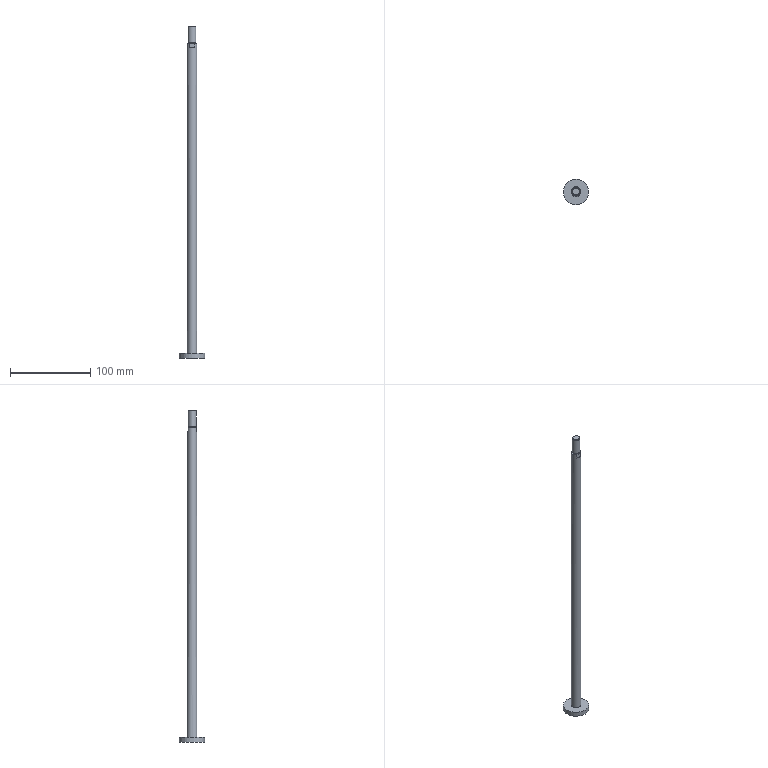Part | STEP file | 163314 DNC-32-320-PPV-A---(FESTO)_HASTE | 1 solid | 13 faces | box 32 x 32 x 415 mm | volume 50245 mm3 | plane 8 | cylinder 3 | cone 2 | commonest cylinder face diameters 10 x1 12 x1 32 x1
STEP:
#1=CARTESIAN_POINT('',(0.,0.,0.));
#2=DIRECTION('',(0.,0.,1.));
#3=DIRECTION('',(1.,0.,0.));
#4=AXIS2_PLACEMENT_3D('',#1,#2,#3);
#5=CARTESIAN_POINT('',(0.,-16.,-361.));
#6=VERTEX_POINT('',#5);
#7=CARTESIAN_POINT('',(0.,0.,-361.));
#8=DIRECTION('',(0.,0.,-1.));
#9=DIRECTION('',(1.,0.,0.));
#10=AXIS2_PLACEMENT_3D('',#7,#8,#9);
#11=CIRCLE('',#10,16.);
#12=CARTESIAN_POINT('',(0.,0.,-364.));
#13=DIRECTION('',(0.,0.,-1.));
#14=DIRECTION('',(0.,-1.,0.));
#15=AXIS2_PLACEMENT_3D('',#12,#13,#14);
#16=CYLINDRICAL_SURFACE('',#15,16.);
#17=CARTESIAN_POINT('',(-1.571,-3.));
#18=DIRECTION('',(1.,0.));
#19=VECTOR('',#18,1.);
#20=LINE('',#17,#19);
#21=(GEOMETRIC_REPRESENTATION_CONTEXT(2)PARAMETRIC_REPRESENTATION_CONTEXT()REPRESENTATION_CONTEXT('',''));
#22=DEFINITIONAL_REPRESENTATION('',(#20),#21);
#23=PCURVE('',#16,#22);
#24=CARTESIAN_POINT('',(0.,9.5,-361.));
#25=DIRECTION('',(0.,0.,1.));
#26=DIRECTION('',(1.,0.,0.));
#27=AXIS2_PLACEMENT_3D('',#24,#25,#26);
#28=PLANE('',#27);
#29=CARTESIAN_POINT('',(16.,-9.5));
#30=CARTESIAN_POINT('',(16.,-37.213));
#31=CARTESIAN_POINT('',(-8.,-23.356));
#32=CARTESIAN_POINT('',(-32.,-9.5));
#33=CARTESIAN_POINT('',(-8.,4.356));
#34=CARTESIAN_POINT('',(16.,18.213));
#35=CARTESIAN_POINT('',(16.,-9.5));
#36=(BOUNDED_CURVE()B_SPLINE_CURVE(2,(#29,#30,#31,#32,#33,#34,#35),.UNSPECIFIED.,.T.,.F.)B_SPLINE_CURVE_WITH_KNOTS((1,2,2,2,2,1),(-2.094,0.,2.094,4.189,6.283,8.378),.UNSPECIFIED.)CURVE()GEOMETRIC_REPRESENTATION_ITEM()RATIONAL_B_SPLINE_CURVE((1.,0.5,1.,0.5,1.,0.5,1.))REPRESENTATION_ITEM(''));
#37=(GEOMETRIC_REPRESENTATION_CONTEXT(2)PARAMETRIC_REPRESENTATION_CONTEXT()REPRESENTATION_CONTEXT('',''));
#38=DEFINITIONAL_REPRESENTATION('',(#36),#37);
#39=PCURVE('',#28,#38);
#40=SURFACE_CURVE('',#11,(#23,#39),.PCURVE_S1.);
#41=EDGE_CURVE('',#6,#6,#40,.T.);
#42=ORIENTED_EDGE('',*,*,#41,.T.);
#43=CARTESIAN_POINT('',(0.,-16.,-367.));
#44=VERTEX_POINT('',#43);
#45=CARTESIAN_POINT('',(0.,-16.,-361.));
#46=CARTESIAN_POINT('',(0.,-16.,-367.));
#47=B_SPLINE_CURVE_WITH_KNOTS('',1,(#45,#46),.UNSPECIFIED.,.F.,.F.,(2,2),(-3.,3.),.PIECEWISE_BEZIER_KNOTS.);
#48=CARTESIAN_POINT('',(6.283,0.));
#49=DIRECTION('',(0.,1.));
#50=VECTOR('',#49,1.);
#51=LINE('',#48,#50);
#52=(GEOMETRIC_REPRESENTATION_CONTEXT(2)PARAMETRIC_REPRESENTATION_CONTEXT()REPRESENTATION_CONTEXT('',''));
#53=DEFINITIONAL_REPRESENTATION('',(#51),#52);
#54=PCURVE('',#16,#53);
#55=CARTESIAN_POINT('',(0.,0.));
#56=DIRECTION('',(0.,1.));
#57=VECTOR('',#56,1.);
#58=LINE('',#55,#57);
#59=(GEOMETRIC_REPRESENTATION_CONTEXT(2)PARAMETRIC_REPRESENTATION_CONTEXT()REPRESENTATION_CONTEXT('',''));
#60=DEFINITIONAL_REPRESENTATION('',(#58),#59);
#61=PCURVE('',#16,#60);
#62=SEAM_CURVE('',#47,(#54,#61),.PCURVE_S1.);
#63=EDGE_CURVE('',#6,#44,#62,.T.);
#64=ORIENTED_EDGE('',*,*,#63,.T.);
#65=CARTESIAN_POINT('',(0.,0.,-367.));
#66=DIRECTION('',(0.,0.,-1.));
#67=DIRECTION('',(1.,0.,0.));
#68=AXIS2_PLACEMENT_3D('',#65,#66,#67);
#69=CIRCLE('',#68,16.);
#70=CARTESIAN_POINT('',(-1.571,3.));
#71=DIRECTION('',(1.,0.));
#72=VECTOR('',#71,1.);
#73=LINE('',#70,#72);
#74=(GEOMETRIC_REPRESENTATION_CONTEXT(2)PARAMETRIC_REPRESENTATION_CONTEXT()REPRESENTATION_CONTEXT('',''));
#75=DEFINITIONAL_REPRESENTATION('',(#73),#74);
#76=PCURVE('',#16,#75);
#77=CARTESIAN_POINT('',(0.,8.,-367.));
#78=DIRECTION('',(0.,0.,-1.));
#79=DIRECTION('',(-1.,0.,0.));
#80=AXIS2_PLACEMENT_3D('',#77,#78,#79);
#81=PLANE('',#80);
#82=CARTESIAN_POINT('',(0.,-8.));
#83=DIRECTION('',(-1.,0.));
#84=AXIS2_PLACEMENT_2D('',#82,#83);
#85=CIRCLE('',#84,16.);
#86=(GEOMETRIC_REPRESENTATION_CONTEXT(2)PARAMETRIC_REPRESENTATION_CONTEXT()REPRESENTATION_CONTEXT('',''));
#87=DEFINITIONAL_REPRESENTATION('',(#85),#86);
#88=PCURVE('',#81,#87);
#89=SURFACE_CURVE('',#69,(#76,#88),.PCURVE_S1.);
#90=EDGE_CURVE('',#44,#44,#89,.T.);
#91=ORIENTED_EDGE('',*,*,#90,.F.);
#92=ORIENTED_EDGE('',*,*,#63,.F.);
#93=EDGE_LOOP('',(#42,#64,#91,#92));
#94=FACE_BOUND('',#93,.T.);
#95=ADVANCED_FACE('',(#94),#16,.T.);
#96=ORIENTED_EDGE('',*,*,#90,.T.);
#97=EDGE_LOOP('',(#96));
#98=FACE_BOUND('',#97,.T.);
#99=ADVANCED_FACE('',(#98),#81,.T.);
#100=ORIENTED_EDGE('',*,*,#41,.F.);
#101=EDGE_LOOP('',(#100));
#102=FACE_BOUND('',#101,.T.);
#103=CARTESIAN_POINT('',(0.,-6.,-361.));
#104=VERTEX_POINT('',#103);
#105=CARTESIAN_POINT('',(0.,0.,-361.));
#106=DIRECTION('',(0.,0.,-1.));
#107=DIRECTION('',(0.,1.,0.));
#108=AXIS2_PLACEMENT_3D('',#105,#106,#107);
#109=CIRCLE('',#108,6.);
#110=CARTESIAN_POINT('',(0.,-3.5));
#111=CARTESIAN_POINT('',(10.392,-3.5));
#112=CARTESIAN_POINT('',(5.196,-12.5));
#113=CARTESIAN_POINT('',(0.,-21.5));
#114=CARTESIAN_POINT('',(-5.196,-12.5));
#115=CARTESIAN_POINT('',(-10.392,-3.5));
#116=CARTESIAN_POINT('',(0.,-3.5));
#117=(BOUNDED_CURVE()B_SPLINE_CURVE(2,(#110,#111,#112,#113,#114,#115,#116),.UNSPECIFIED.,.T.,.F.)B_SPLINE_CURVE_WITH_KNOTS((1,2,2,2,2,1),(-2.094,0.,2.094,4.189,6.283,8.378),.UNSPECIFIED.)CURVE()GEOMETRIC_REPRESENTATION_ITEM()RATIONAL_B_SPLINE_CURVE((1.,0.5,1.,0.5,1.,0.5,1.))REPRESENTATION_ITEM(''));
#118=(GEOMETRIC_REPRESENTATION_CONTEXT(2)PARAMETRIC_REPRESENTATION_CONTEXT()REPRESENTATION_CONTEXT('',''));
#119=DEFINITIONAL_REPRESENTATION('',(#117),#118);
#120=PCURVE('',#28,#119);
#121=CARTESIAN_POINT('',(0.,0.,-170.45));
#122=DIRECTION('',(0.,0.,-1.));
#123=DIRECTION('',(0.,-1.,0.));
#124=AXIS2_PLACEMENT_3D('',#121,#122,#123);
#125=CYLINDRICAL_SURFACE('',#124,6.);
#126=CARTESIAN_POINT('',(-3.142,190.55));
#127=DIRECTION('',(1.,0.));
#128=VECTOR('',#127,1.);
#129=LINE('',#126,#128);
#130=(GEOMETRIC_REPRESENTATION_CONTEXT(2)PARAMETRIC_REPRESENTATION_CONTEXT()REPRESENTATION_CONTEXT('',''));
#131=DEFINITIONAL_REPRESENTATION('',(#129),#130);
#132=PCURVE('',#125,#131);
#133=SURFACE_CURVE('',#109,(#120,#132),.PCURVE_S1.);
#134=EDGE_CURVE('',#104,#104,#133,.T.);
#135=ORIENTED_EDGE('',*,*,#134,.T.);
#136=EDGE_LOOP('',(#135));
#137=FACE_BOUND('',#136,.T.);
#138=ADVANCED_FACE('',(#102,#137),#28,.T.);
#139=CARTESIAN_POINT('',(3.317,-5.,21.));
#140=VERTEX_POINT('',#139);
#141=CARTESIAN_POINT('',(0.,-6.,21.));
#142=VERTEX_POINT('',#141);
#143=CARTESIAN_POINT('',(0.,0.,21.));
#144=DIRECTION('',(0.,0.,-1.));
#145=DIRECTION('',(-0.5528,-0.8333,0.));
#146=AXIS2_PLACEMENT_3D('',#143,#144,#145);
#147=CIRCLE('',#146,6.);
#148=CARTESIAN_POINT('',(0.5857,-191.45));
#149=DIRECTION('',(1.,0.000000001));
#150=VECTOR('',#149,1.);
#151=LINE('',#148,#150);
#152=(GEOMETRIC_REPRESENTATION_CONTEXT(2)PARAMETRIC_REPRESENTATION_CONTEXT()REPRESENTATION_CONTEXT('',''));
#153=DEFINITIONAL_REPRESENTATION('',(#151),#152);
#154=PCURVE('',#125,#153);
#155=CARTESIAN_POINT('',(0.,0.,21.));
#156=DIRECTION('',(0.,0.,1.));
#157=DIRECTION('',(1.,0.,0.));
#158=AXIS2_PLACEMENT_3D('',#155,#156,#157);
#159=PLANE('',#158);
#160=CARTESIAN_POINT('',(-3.317,-5.));
#161=CARTESIAN_POINT('',(-11.977,0.7446));
#162=CARTESIAN_POINT('',(-2.672,5.372));
#163=CARTESIAN_POINT('',(6.633,10.));
#164=CARTESIAN_POINT('',(5.988,-0.3723));
#165=CARTESIAN_POINT('',(5.344,-10.745));
#166=CARTESIAN_POINT('',(-3.317,-5.));
#167=(BOUNDED_CURVE()B_SPLINE_CURVE(2,(#160,#161,#162,#163,#164,#165,#166),.UNSPECIFIED.,.T.,.F.)B_SPLINE_CURVE_WITH_KNOTS((1,2,2,2,2,1),(-2.094,0.,2.094,4.189,6.283,8.378),.UNSPECIFIED.)CURVE()GEOMETRIC_REPRESENTATION_ITEM()RATIONAL_B_SPLINE_CURVE((1.,0.5,1.,0.5,1.,0.5,1.))REPRESENTATION_ITEM(''));
#168=(GEOMETRIC_REPRESENTATION_CONTEXT(2)PARAMETRIC_REPRESENTATION_CONTEXT()REPRESENTATION_CONTEXT('',''));
#169=DEFINITIONAL_REPRESENTATION('',(#167),#168);
#170=PCURVE('',#159,#169);
#171=SURFACE_CURVE('',#147,(#154,#170),.PCURVE_S1.);
#172=EDGE_CURVE('',#140,#142,#171,.T.);
#173=ORIENTED_EDGE('',*,*,#172,.T.);
#174=CARTESIAN_POINT('',(0.,-6.,21.));
#175=CARTESIAN_POINT('',(0.,-6.,-361.));
#176=B_SPLINE_CURVE_WITH_KNOTS('',1,(#174,#175),.UNSPECIFIED.,.F.,.F.,(2,2),(-191.45,190.55),.PIECEWISE_BEZIER_KNOTS.);
#177=CARTESIAN_POINT('',(6.283,0.));
#178=DIRECTION('',(0.,1.));
#179=VECTOR('',#178,1.);
#180=LINE('',#177,#179);
#181=(GEOMETRIC_REPRESENTATION_CONTEXT(2)PARAMETRIC_REPRESENTATION_CONTEXT()REPRESENTATION_CONTEXT('',''));
#182=DEFINITIONAL_REPRESENTATION('',(#180),#181);
#183=PCURVE('',#125,#182);
#184=CARTESIAN_POINT('',(0.,0.));
#185=DIRECTION('',(0.,1.));
#186=VECTOR('',#185,1.);
#187=LINE('',#184,#186);
#188=(GEOMETRIC_REPRESENTATION_CONTEXT(2)PARAMETRIC_REPRESENTATION_CONTEXT()REPRESENTATION_CONTEXT('',''));
#189=DEFINITIONAL_REPRESENTATION('',(#187),#188);
#190=PCURVE('',#125,#189);
#191=SEAM_CURVE('',#176,(#183,#190),.PCURVE_S1.);
#192=EDGE_CURVE('',#142,#104,#191,.T.);
#193=ORIENTED_EDGE('',*,*,#192,.T.);
#194=ORIENTED_EDGE('',*,*,#134,.F.);
#195=ORIENTED_EDGE('',*,*,#192,.F.);
#196=CARTESIAN_POINT('',(-3.317,-5.,21.));
#197=VERTEX_POINT('',#196);
#198=CARTESIAN_POINT('',(0.,0.,21.));
#199=DIRECTION('',(0.,0.,-1.));
#200=DIRECTION('',(-0.5528,-0.8333,0.));
#201=AXIS2_PLACEMENT_3D('',#198,#199,#200);
#202=CIRCLE('',#201,6.);
#203=CARTESIAN_POINT('',(-5.697,-191.45));
#204=DIRECTION('',(1.,0.000000001));
#205=VECTOR('',#204,1.);
#206=LINE('',#203,#205);
#207=(GEOMETRIC_REPRESENTATION_CONTEXT(2)PARAMETRIC_REPRESENTATION_CONTEXT()REPRESENTATION_CONTEXT('',''));
#208=DEFINITIONAL_REPRESENTATION('',(#206),#207);
#209=PCURVE('',#125,#208);
#210=CARTESIAN_POINT('',(-3.317,-5.));
#211=CARTESIAN_POINT('',(-11.977,0.7446));
#212=CARTESIAN_POINT('',(-2.672,5.372));
#213=CARTESIAN_POINT('',(6.633,10.));
#214=CARTESIAN_POINT('',(5.988,-0.3723));
#215=CARTESIAN_POINT('',(5.344,-10.745));
#216=CARTESIAN_POINT('',(-3.317,-5.));
#217=(BOUNDED_CURVE()B_SPLINE_CURVE(2,(#210,#211,#212,#213,#214,#215,#216),.UNSPECIFIED.,.T.,.F.)B_SPLINE_CURVE_WITH_KNOTS((1,2,2,2,2,1),(-2.094,0.,2.094,4.189,6.283,8.378),.UNSPECIFIED.)CURVE()GEOMETRIC_REPRESENTATION_ITEM()RATIONAL_B_SPLINE_CURVE((1.,0.5,1.,0.5,1.,0.5,1.))REPRESENTATION_ITEM(''));
#218=(GEOMETRIC_REPRESENTATION_CONTEXT(2)PARAMETRIC_REPRESENTATION_CONTEXT()REPRESENTATION_CONTEXT('',''));
#219=DEFINITIONAL_REPRESENTATION('',(#217),#218);
#220=PCURVE('',#159,#219);
#221=SURFACE_CURVE('',#202,(#209,#220),.PCURVE_S1.);
#222=EDGE_CURVE('',#142,#197,#221,.T.);
#223=ORIENTED_EDGE('',*,*,#222,.T.);
#224=CARTESIAN_POINT('',(-3.317,-5.,26.));
#225=VERTEX_POINT('',#224);
#226=CARTESIAN_POINT('',(-3.317,-5.,26.));
#227=DIRECTION('',(0.,0.,-1.));
#228=VECTOR('',#227,1.);
#229=LINE('',#226,#228);
#230=CARTESIAN_POINT('',(0.5857,-196.45));
#231=DIRECTION('',(0.,1.));
#232=VECTOR('',#231,1.);
#233=LINE('',#230,#232);
#234=(GEOMETRIC_REPRESENTATION_CONTEXT(2)PARAMETRIC_REPRESENTATION_CONTEXT()REPRESENTATION_CONTEXT('',''));
#235=DEFINITIONAL_REPRESENTATION('',(#233),#234);
#236=PCURVE('',#125,#235);
#237=CARTESIAN_POINT('',(12.,-5.,31.));
#238=DIRECTION('',(0.,1.,0.));
#239=DIRECTION('',(0.,0.,1.));
#240=AXIS2_PLACEMENT_3D('',#237,#238,#239);
#241=PLANE('',#240);
#242=CARTESIAN_POINT('',(-5.,-15.317));
#243=DIRECTION('',(-1.,0.));
#244=VECTOR('',#243,1.);
#245=LINE('',#242,#244);
#246=(GEOMETRIC_REPRESENTATION_CONTEXT(2)PARAMETRIC_REPRESENTATION_CONTEXT()REPRESENTATION_CONTEXT('',''));
#247=DEFINITIONAL_REPRESENTATION('',(#245),#246);
#248=PCURVE('',#241,#247);
#249=SURFACE_CURVE('',#229,(#236,#248),.PCURVE_S1.);
#250=EDGE_CURVE('',#225,#197,#249,.T.);
#251=ORIENTED_EDGE('',*,*,#250,.F.);
#252=CARTESIAN_POINT('',(-3.317,5.,26.));
#253=VERTEX_POINT('',#252);
#254=CARTESIAN_POINT('',(0.,0.,26.));
#255=DIRECTION('',(0.,0.,-1.));
#256=DIRECTION('',(1.,0.,0.));
#257=AXIS2_PLACEMENT_3D('',#254,#255,#256);
#258=CIRCLE('',#257,6.);
#259=CARTESIAN_POINT('',(-1.571,-196.45));
#260=DIRECTION('',(1.,0.));
#261=VECTOR('',#260,1.);
#262=LINE('',#259,#261);
#263=(GEOMETRIC_REPRESENTATION_CONTEXT(2)PARAMETRIC_REPRESENTATION_CONTEXT()REPRESENTATION_CONTEXT('',''));
#264=DEFINITIONAL_REPRESENTATION('',(#262),#263);
#265=PCURVE('',#125,#264);
#266=CARTESIAN_POINT('',(0.,3.,26.));
#267=DIRECTION('',(0.,0.,1.));
#268=DIRECTION('',(1.,0.,0.));
#269=AXIS2_PLACEMENT_3D('',#266,#267,#268);
#270=PLANE('',#269);
#271=CARTESIAN_POINT('',(6.,-3.));
#272=CARTESIAN_POINT('',(6.,-13.392));
#273=CARTESIAN_POINT('',(-3.,-8.196));
#274=CARTESIAN_POINT('',(-12.,-3.));
#275=CARTESIAN_POINT('',(-3.,2.196));
#276=CARTESIAN_POINT('',(6.,7.392));
#277=CARTESIAN_POINT('',(6.,-3.));
#278=(BOUNDED_CURVE()B_SPLINE_CURVE(2,(#271,#272,#273,#274,#275,#276,#277),.UNSPECIFIED.,.T.,.F.)B_SPLINE_CURVE_WITH_KNOTS((1,2,2,2,2,1),(-2.094,0.,2.094,4.189,6.283,8.378),.UNSPECIFIED.)CURVE()GEOMETRIC_REPRESENTATION_ITEM()RATIONAL_B_SPLINE_CURVE((1.,0.5,1.,0.5,1.,0.5,1.))REPRESENTATION_ITEM(''));
#279=(GEOMETRIC_REPRESENTATION_CONTEXT(2)PARAMETRIC_REPRESENTATION_CONTEXT()REPRESENTATION_CONTEXT('',''));
#280=DEFINITIONAL_REPRESENTATION('',(#278),#279);
#281=PCURVE('',#270,#280);
#282=SURFACE_CURVE('',#258,(#265,#281),.PCURVE_S1.);
#283=EDGE_CURVE('',#225,#253,#282,.T.);
#284=ORIENTED_EDGE('',*,*,#283,.T.);
#285=CARTESIAN_POINT('',(-3.317,5.,21.));
#286=VERTEX_POINT('',#285);
#287=CARTESIAN_POINT('',(-3.317,5.,26.));
#288=DIRECTION('',(0.,0.,-1.));
#289=VECTOR('',#288,1.);
#290=LINE('',#287,#289);
#291=CARTESIAN_POINT('',(2.556,-196.45));
#292=DIRECTION('',(0.,1.));
#293=VECTOR('',#292,1.);
#294=LINE('',#291,#293);
#295=(GEOMETRIC_REPRESENTATION_CONTEXT(2)PARAMETRIC_REPRESENTATION_CONTEXT()REPRESENTATION_CONTEXT('',''));
#296=DEFINITIONAL_REPRESENTATION('',(#294),#295);
#297=PCURVE('',#125,#296);
#298=CARTESIAN_POINT('',(-12.,5.,31.));
#299=DIRECTION('',(0.,-1.,0.));
#300=DIRECTION('',(0.,0.,-1.));
#301=AXIS2_PLACEMENT_3D('',#298,#299,#300);
#302=PLANE('',#301);
#303=CARTESIAN_POINT('',(5.,8.683));
#304=DIRECTION('',(1.,0.));
#305=VECTOR('',#304,1.);
#306=LINE('',#303,#305);
#307=(GEOMETRIC_REPRESENTATION_CONTEXT(2)PARAMETRIC_REPRESENTATION_CONTEXT()REPRESENTATION_CONTEXT('',''));
#308=DEFINITIONAL_REPRESENTATION('',(#306),#307);
#309=PCURVE('',#302,#308);
#310=SURFACE_CURVE('',#290,(#297,#309),.PCURVE_S1.);
#311=EDGE_CURVE('',#253,#286,#310,.T.);
#312=ORIENTED_EDGE('',*,*,#311,.T.);
#313=CARTESIAN_POINT('',(3.317,5.,21.));
#314=VERTEX_POINT('',#313);
#315=CARTESIAN_POINT('',(0.,0.,21.));
#316=DIRECTION('',(0.,0.,-1.));
#317=DIRECTION('',(1.,0.,0.));
#318=AXIS2_PLACEMENT_3D('',#315,#316,#317);
#319=CIRCLE('',#318,6.);
#320=CARTESIAN_POINT('',(-1.571,-191.45));
#321=DIRECTION('',(1.,0.));
#322=VECTOR('',#321,1.);
#323=LINE('',#320,#322);
#324=(GEOMETRIC_REPRESENTATION_CONTEXT(2)PARAMETRIC_REPRESENTATION_CONTEXT()REPRESENTATION_CONTEXT('',''));
#325=DEFINITIONAL_REPRESENTATION('',(#323),#324);
#326=PCURVE('',#125,#325);
#327=CARTESIAN_POINT('',(0.,0.,21.));
#328=DIRECTION('',(0.,0.,1.));
#329=DIRECTION('',(1.,0.,0.));
#330=AXIS2_PLACEMENT_3D('',#327,#328,#329);
#331=PLANE('',#330);
#332=CARTESIAN_POINT('',(6.,0.));
#333=CARTESIAN_POINT('',(6.,-10.392));
#334=CARTESIAN_POINT('',(-3.,-5.196));
#335=CARTESIAN_POINT('',(-12.,0.));
#336=CARTESIAN_POINT('',(-3.,5.196));
#337=CARTESIAN_POINT('',(6.,10.392));
#338=CARTESIAN_POINT('',(6.,0.));
#339=(BOUNDED_CURVE()B_SPLINE_CURVE(2,(#332,#333,#334,#335,#336,#337,#338),.UNSPECIFIED.,.T.,.F.)B_SPLINE_CURVE_WITH_KNOTS((1,2,2,2,2,1),(-2.094,0.,2.094,4.189,6.283,8.378),.UNSPECIFIED.)CURVE()GEOMETRIC_REPRESENTATION_ITEM()RATIONAL_B_SPLINE_CURVE((1.,0.5,1.,0.5,1.,0.5,1.))REPRESENTATION_ITEM(''));
#340=(GEOMETRIC_REPRESENTATION_CONTEXT(2)PARAMETRIC_REPRESENTATION_CONTEXT()REPRESENTATION_CONTEXT('',''));
#341=DEFINITIONAL_REPRESENTATION('',(#339),#340);
#342=PCURVE('',#331,#341);
#343=SURFACE_CURVE('',#319,(#326,#342),.PCURVE_S1.);
#344=EDGE_CURVE('',#286,#314,#343,.T.);
#345=ORIENTED_EDGE('',*,*,#344,.T.);
#346=CARTESIAN_POINT('',(3.317,5.,26.));
#347=VERTEX_POINT('',#346);
#348=CARTESIAN_POINT('',(3.317,5.,26.));
#349=DIRECTION('',(0.,0.,-1.));
#350=VECTOR('',#349,1.);
#351=LINE('',#348,#350);
#352=CARTESIAN_POINT('',(3.727,-196.45));
#353=DIRECTION('',(0.,1.));
#354=VECTOR('',#353,1.);
#355=LINE('',#352,#354);
#356=(GEOMETRIC_REPRESENTATION_CONTEXT(2)PARAMETRIC_REPRESENTATION_CONTEXT()REPRESENTATION_CONTEXT('',''));
#357=DEFINITIONAL_REPRESENTATION('',(#355),#356);
#358=PCURVE('',#125,#357);
#359=CARTESIAN_POINT('',(5.,15.317));
#360=DIRECTION('',(1.,0.));
#361=VECTOR('',#360,1.);
#362=LINE('',#359,#361);
#363=(GEOMETRIC_REPRESENTATION_CONTEXT(2)PARAMETRIC_REPRESENTATION_CONTEXT()REPRESENTATION_CONTEXT('',''));
#364=DEFINITIONAL_REPRESENTATION('',(#362),#363);
#365=PCURVE('',#302,#364);
#366=SURFACE_CURVE('',#351,(#358,#365),.PCURVE_S1.);
#367=EDGE_CURVE('',#347,#314,#366,.T.);
#368=ORIENTED_EDGE('',*,*,#367,.F.);
#369=CARTESIAN_POINT('',(3.317,-5.,26.));
#370=VERTEX_POINT('',#369);
#371=CARTESIAN_POINT('',(0.,0.,26.));
#372=DIRECTION('',(0.,0.,-1.));
#373=DIRECTION('',(1.,0.,0.));
#374=AXIS2_PLACEMENT_3D('',#371,#372,#373);
#375=CIRCLE('',#374,6.);
#376=CARTESIAN_POINT('',(-1.571,-196.45));
#377=DIRECTION('',(1.,0.));
#378=VECTOR('',#377,1.);
#379=LINE('',#376,#378);
#380=(GEOMETRIC_REPRESENTATION_CONTEXT(2)PARAMETRIC_REPRESENTATION_CONTEXT()REPRESENTATION_CONTEXT('',''));
#381=DEFINITIONAL_REPRESENTATION('',(#379),#380);
#382=PCURVE('',#125,#381);
#383=CARTESIAN_POINT('',(6.,-3.));
#384=CARTESIAN_POINT('',(6.,-13.392));
#385=CARTESIAN_POINT('',(-3.,-8.196));
#386=CARTESIAN_POINT('',(-12.,-3.));
#387=CARTESIAN_POINT('',(-3.,2.196));
#388=CARTESIAN_POINT('',(6.,7.392));
#389=CARTESIAN_POINT('',(6.,-3.));
#390=(BOUNDED_CURVE()B_SPLINE_CURVE(2,(#383,#384,#385,#386,#387,#388,#389),.UNSPECIFIED.,.T.,.F.)B_SPLINE_CURVE_WITH_KNOTS((1,2,2,2,2,1),(-2.094,0.,2.094,4.189,6.283,8.378),.UNSPECIFIED.)CURVE()GEOMETRIC_REPRESENTATION_ITEM()RATIONAL_B_SPLINE_CURVE((1.,0.5,1.,0.5,1.,0.5,1.))REPRESENTATION_ITEM(''));
#391=(GEOMETRIC_REPRESENTATION_CONTEXT(2)PARAMETRIC_REPRESENTATION_CONTEXT()REPRESENTATION_CONTEXT('',''));
#392=DEFINITIONAL_REPRESENTATION('',(#390),#391);
#393=PCURVE('',#270,#392);
#394=SURFACE_CURVE('',#375,(#382,#393),.PCURVE_S1.);
#395=EDGE_CURVE('',#347,#370,#394,.T.);
#396=ORIENTED_EDGE('',*,*,#395,.T.);
#397=CARTESIAN_POINT('',(3.317,-5.,26.));
#398=DIRECTION('',(0.,0.,-1.));
#399=VECTOR('',#398,1.);
#400=LINE('',#397,#399);
#401=CARTESIAN_POINT('',(5.697,-196.45));
#402=DIRECTION('',(0.,1.));
#403=VECTOR('',#402,1.);
#404=LINE('',#401,#403);
#405=(GEOMETRIC_REPRESENTATION_CONTEXT(2)PARAMETRIC_REPRESENTATION_CONTEXT()REPRESENTATION_CONTEXT('',''));
#406=DEFINITIONAL_REPRESENTATION('',(#404),#405);
#407=PCURVE('',#125,#406);
#408=CARTESIAN_POINT('',(-5.,-8.683));
#409=DIRECTION('',(-1.,0.));
#410=VECTOR('',#409,1.);
#411=LINE('',#408,#410);
#412=(GEOMETRIC_REPRESENTATION_CONTEXT(2)PARAMETRIC_REPRESENTATION_CONTEXT()REPRESENTATION_CONTEXT('',''));
#413=DEFINITIONAL_REPRESENTATION('',(#411),#412);
#414=PCURVE('',#241,#413);
#415=SURFACE_CURVE('',#400,(#407,#414),.PCURVE_S1.);
#416=EDGE_CURVE('',#370,#140,#415,.T.);
#417=ORIENTED_EDGE('',*,*,#416,.T.);
#418=EDGE_LOOP('',(#173,#193,#194,#195,#223,#251,#284,#312,#345,#368,#396,#417));
#419=FACE_BOUND('',#418,.T.);
#420=ADVANCED_FACE('',(#419),#125,.T.);
#421=ORIENTED_EDGE('',*,*,#172,.F.);
#422=CARTESIAN_POINT('',(3.317,-5.,21.));
#423=DIRECTION('',(-1.,0.,0.));
#424=VECTOR('',#423,1.);
#425=LINE('',#422,#424);
#426=CARTESIAN_POINT('',(3.317,-5.));
#427=DIRECTION('',(-1.,0.));
#428=VECTOR('',#427,1.);
#429=LINE('',#426,#428);
#430=(GEOMETRIC_REPRESENTATION_CONTEXT(2)PARAMETRIC_REPRESENTATION_CONTEXT()REPRESENTATION_CONTEXT('',''));
#431=DEFINITIONAL_REPRESENTATION('',(#429),#430);
#432=PCURVE('',#159,#431);
#433=CARTESIAN_POINT('',(-10.,-8.683));
#434=DIRECTION('',(0.,-1.));
#435=VECTOR('',#434,1.);
#436=LINE('',#433,#435);
#437=(GEOMETRIC_REPRESENTATION_CONTEXT(2)PARAMETRIC_REPRESENTATION_CONTEXT()REPRESENTATION_CONTEXT('',''));
#438=DEFINITIONAL_REPRESENTATION('',(#436),#437);
#439=PCURVE('',#241,#438);
#440=SURFACE_CURVE('',#425,(#432,#439),.PCURVE_S1.);
#441=EDGE_CURVE('',#140,#197,#440,.T.);
#442=ORIENTED_EDGE('',*,*,#441,.T.);
#443=ORIENTED_EDGE('',*,*,#222,.F.);
#444=EDGE_LOOP('',(#421,#442,#443));
#445=FACE_BOUND('',#444,.T.);
#446=ADVANCED_FACE('',(#445),#159,.T.);
#447=ORIENTED_EDGE('',*,*,#250,.T.);
#448=ORIENTED_EDGE('',*,*,#441,.F.);
#449=ORIENTED_EDGE('',*,*,#416,.F.);
#450=CARTESIAN_POINT('',(-3.317,-5.,26.));
#451=DIRECTION('',(1.,0.,0.));
#452=VECTOR('',#451,1.);
#453=LINE('',#450,#452);
#454=CARTESIAN_POINT('',(-5.,-15.317));
#455=DIRECTION('',(0.,1.));
#456=VECTOR('',#455,1.);
#457=LINE('',#454,#456);
#458=(GEOMETRIC_REPRESENTATION_CONTEXT(2)PARAMETRIC_REPRESENTATION_CONTEXT()REPRESENTATION_CONTEXT('',''));
#459=DEFINITIONAL_REPRESENTATION('',(#457),#458);
#460=PCURVE('',#241,#459);
#461=CARTESIAN_POINT('',(-3.317,-8.));
#462=DIRECTION('',(1.,0.));
#463=VECTOR('',#462,1.);
#464=LINE('',#461,#463);
#465=(GEOMETRIC_REPRESENTATION_CONTEXT(2)PARAMETRIC_REPRESENTATION_CONTEXT()REPRESENTATION_CONTEXT('',''));
#466=DEFINITIONAL_REPRESENTATION('',(#464),#465);
#467=PCURVE('',#270,#466);
#468=SURFACE_CURVE('',#453,(#460,#467),.PCURVE_S1.);
#469=EDGE_CURVE('',#225,#370,#468,.T.);
#470=ORIENTED_EDGE('',*,*,#469,.F.);
#471=EDGE_LOOP('',(#447,#448,#449,#470));
#472=FACE_BOUND('',#471,.T.);
#473=ADVANCED_FACE('',(#472),#241,.F.);
#474=ORIENTED_EDGE('',*,*,#469,.T.);
#475=ORIENTED_EDGE('',*,*,#395,.F.);
#476=CARTESIAN_POINT('',(3.317,5.,26.));
#477=DIRECTION('',(-1.,0.,0.));
#478=VECTOR('',#477,1.);
#479=LINE('',#476,#478);
#480=CARTESIAN_POINT('',(3.317,2.));
#481=DIRECTION('',(-1.,0.));
#482=VECTOR('',#481,1.);
#483=LINE('',#480,#482);
#484=(GEOMETRIC_REPRESENTATION_CONTEXT(2)PARAMETRIC_REPRESENTATION_CONTEXT()REPRESENTATION_CONTEXT('',''));
#485=DEFINITIONAL_REPRESENTATION('',(#483),#484);
#486=PCURVE('',#270,#485);
#487=CARTESIAN_POINT('',(5.,15.317));
#488=DIRECTION('',(0.,-1.));
#489=VECTOR('',#488,1.);
#490=LINE('',#487,#489);
#491=(GEOMETRIC_REPRESENTATION_CONTEXT(2)PARAMETRIC_REPRESENTATION_CONTEXT()REPRESENTATION_CONTEXT('',''));
#492=DEFINITIONAL_REPRESENTATION('',(#490),#491);
#493=PCURVE('',#302,#492);
#494=SURFACE_CURVE('',#479,(#486,#493),.PCURVE_S1.);
#495=EDGE_CURVE('',#347,#253,#494,.T.);
#496=ORIENTED_EDGE('',*,*,#495,.T.);
#497=ORIENTED_EDGE('',*,*,#283,.F.);
#498=EDGE_LOOP('',(#474,#475,#496,#497));
#499=FACE_BOUND('',#498,.T.);
#500=CARTESIAN_POINT('',(0.,-4.138,26.));
#501=VERTEX_POINT('',#500);
#502=CARTESIAN_POINT('',(0.,0.,26.));
#503=DIRECTION('',(0.,0.,-1.));
#504=DIRECTION('',(0.,1.,0.));
#505=AXIS2_PLACEMENT_3D('',#502,#503,#504);
#506=CIRCLE('',#505,4.138);
#507=CARTESIAN_POINT('',(0.,1.138));
#508=CARTESIAN_POINT('',(7.167,1.138));
#509=CARTESIAN_POINT('',(3.583,-5.069));
#510=CARTESIAN_POINT('',(0.,-11.275));
#511=CARTESIAN_POINT('',(-3.583,-5.069));
#512=CARTESIAN_POINT('',(-7.167,1.138));
#513=CARTESIAN_POINT('',(0.,1.138));
#514=(BOUNDED_CURVE()B_SPLINE_CURVE(2,(#507,#508,#509,#510,#511,#512,#513),.UNSPECIFIED.,.T.,.F.)B_SPLINE_CURVE_WITH_KNOTS((1,2,2,2,2,1),(-2.094,0.,2.094,4.189,6.283,8.378),.UNSPECIFIED.)CURVE()GEOMETRIC_REPRESENTATION_ITEM()RATIONAL_B_SPLINE_CURVE((1.,0.5,1.,0.5,1.,0.5,1.))REPRESENTATION_ITEM(''));
#515=(GEOMETRIC_REPRESENTATION_CONTEXT(2)PARAMETRIC_REPRESENTATION_CONTEXT()REPRESENTATION_CONTEXT('',''));
#516=DEFINITIONAL_REPRESENTATION('',(#514),#515);
#517=PCURVE('',#270,#516);
#518=CARTESIAN_POINT('',(0.,0.,26.697));
#519=DIRECTION('',(0.,0.,1.));
#520=DIRECTION('',(0.,1.,0.));
#521=AXIS2_PLACEMENT_3D('',#518,#519,#520);
#522=CONICAL_SURFACE('',#521,4.54,0.5236);
#523=CARTESIAN_POINT('',(12.566,-0.6967));
#524=DIRECTION('',(-1.,0.));
#525=VECTOR('',#524,1.);
#526=LINE('',#523,#525);
#527=(GEOMETRIC_REPRESENTATION_CONTEXT(2)PARAMETRIC_REPRESENTATION_CONTEXT()REPRESENTATION_CONTEXT('',''));
#528=DEFINITIONAL_REPRESENTATION('',(#526),#527);
#529=PCURVE('',#522,#528);
#530=SURFACE_CURVE('',#506,(#517,#529),.PCURVE_S1.);
#531=EDGE_CURVE('',#501,#501,#530,.T.);
#532=ORIENTED_EDGE('',*,*,#531,.T.);
#533=EDGE_LOOP('',(#532));
#534=FACE_BOUND('',#533,.T.);
#535=ADVANCED_FACE('',(#499,#534),#270,.T.);
#536=ORIENTED_EDGE('',*,*,#311,.F.);
#537=ORIENTED_EDGE('',*,*,#495,.F.);
#538=ORIENTED_EDGE('',*,*,#367,.T.);
#539=CARTESIAN_POINT('',(-3.317,5.,21.));
#540=DIRECTION('',(1.,0.,0.));
#541=VECTOR('',#540,1.);
#542=LINE('',#539,#541);
#543=CARTESIAN_POINT('',(10.,8.683));
#544=DIRECTION('',(0.,1.));
#545=VECTOR('',#544,1.);
#546=LINE('',#543,#545);
#547=(GEOMETRIC_REPRESENTATION_CONTEXT(2)PARAMETRIC_REPRESENTATION_CONTEXT()REPRESENTATION_CONTEXT('',''));
#548=DEFINITIONAL_REPRESENTATION('',(#546),#547);
#549=PCURVE('',#302,#548);
#550=CARTESIAN_POINT('',(-3.317,5.));
#551=DIRECTION('',(1.,0.));
#552=VECTOR('',#551,1.);
#553=LINE('',#550,#552);
#554=(GEOMETRIC_REPRESENTATION_CONTEXT(2)PARAMETRIC_REPRESENTATION_CONTEXT()REPRESENTATION_CONTEXT('',''));
#555=DEFINITIONAL_REPRESENTATION('',(#553),#554);
#556=PCURVE('',#331,#555);
#557=SURFACE_CURVE('',#542,(#549,#556),.PCURVE_S1.);
#558=EDGE_CURVE('',#286,#314,#557,.T.);
#559=ORIENTED_EDGE('',*,*,#558,.F.);
#560=EDGE_LOOP('',(#536,#537,#538,#559));
#561=FACE_BOUND('',#560,.T.);
#562=ADVANCED_FACE('',(#561),#302,.F.);
#563=ORIENTED_EDGE('',*,*,#344,.F.);
#564=ORIENTED_EDGE('',*,*,#558,.T.);
#565=EDGE_LOOP('',(#563,#564));
#566=FACE_BOUND('',#565,.T.);
#567=ADVANCED_FACE('',(#566),#331,.T.);
#568=CARTESIAN_POINT('',(0.,-5.,27.493));
#569=VERTEX_POINT('',#568);
#570=CARTESIAN_POINT('',(0.,0.,27.493));
#571=DIRECTION('',(0.,0.,1.));
#572=DIRECTION('',(1.,0.,0.));
#573=AXIS2_PLACEMENT_3D('',#570,#571,#572);
#574=CIRCLE('',#573,5.);
#575=CARTESIAN_POINT('',(-1.571,0.7967));
#576=DIRECTION('',(1.,0.));
#577=VECTOR('',#576,1.);
#578=LINE('',#575,#577);
#579=(GEOMETRIC_REPRESENTATION_CONTEXT(2)PARAMETRIC_REPRESENTATION_CONTEXT()REPRESENTATION_CONTEXT('',''));
#580=DEFINITIONAL_REPRESENTATION('',(#578),#579);
#581=PCURVE('',#522,#580);
#582=CARTESIAN_POINT('',(0.,0.,37.287));
#583=DIRECTION('',(0.,0.,-1.));
#584=DIRECTION('',(0.,-1.,0.));
#585=AXIS2_PLACEMENT_3D('',#582,#583,#584);
#586=CYLINDRICAL_SURFACE('',#585,5.);
#587=CARTESIAN_POINT('',(10.996,9.793));
#588=DIRECTION('',(-1.,0.));
#589=VECTOR('',#588,1.);
#590=LINE('',#587,#589);
#591=(GEOMETRIC_REPRESENTATION_CONTEXT(2)PARAMETRIC_REPRESENTATION_CONTEXT()REPRESENTATION_CONTEXT('',''));
#592=DEFINITIONAL_REPRESENTATION('',(#590),#591);
#593=PCURVE('',#586,#592);
#594=SURFACE_CURVE('',#574,(#581,#593),.PCURVE_S1.);
#595=EDGE_CURVE('',#569,#569,#594,.T.);
#596=ORIENTED_EDGE('',*,*,#595,.F.);
#597=CARTESIAN_POINT('',(0.,-4.138,26.));
#598=CARTESIAN_POINT('',(0.,-5.,27.493));
#599=B_SPLINE_CURVE_WITH_KNOTS('',1,(#597,#598),.UNSPECIFIED.,.F.,.F.,(2,2),(-0.8045,0.92),.PIECEWISE_BEZIER_KNOTS.);
#600=CARTESIAN_POINT('',(3.142,0.));
#601=DIRECTION('',(0.,1.));
#602=VECTOR('',#601,1.);
#603=LINE('',#600,#602);
#604=(GEOMETRIC_REPRESENTATION_CONTEXT(2)PARAMETRIC_REPRESENTATION_CONTEXT()REPRESENTATION_CONTEXT('',''));
#605=DEFINITIONAL_REPRESENTATION('',(#603),#604);
#606=PCURVE('',#522,#605);
#607=CARTESIAN_POINT('',(9.425,0.));
#608=DIRECTION('',(0.,1.));
#609=VECTOR('',#608,1.);
#610=LINE('',#607,#609);
#611=(GEOMETRIC_REPRESENTATION_CONTEXT(2)PARAMETRIC_REPRESENTATION_CONTEXT()REPRESENTATION_CONTEXT('',''));
#612=DEFINITIONAL_REPRESENTATION('',(#610),#611);
#613=PCURVE('',#522,#612);
#614=SEAM_CURVE('',#599,(#606,#613),.PCURVE_S1.);
#615=EDGE_CURVE('',#501,#569,#614,.T.);
#616=ORIENTED_EDGE('',*,*,#615,.F.);
#617=ORIENTED_EDGE('',*,*,#531,.F.);
#618=ORIENTED_EDGE('',*,*,#615,.T.);
#619=EDGE_LOOP('',(#596,#616,#617,#618));
#620=FACE_BOUND('',#619,.T.);
#621=ADVANCED_FACE('',(#620),#522,.T.);
#622=CARTESIAN_POINT('',(0.,-5.,47.08));
#623=VERTEX_POINT('',#622);
#624=CARTESIAN_POINT('',(0.,0.,47.08));
#625=DIRECTION('',(0.,0.,-1.));
#626=DIRECTION('',(1.,0.,0.));
#627=AXIS2_PLACEMENT_3D('',#624,#625,#626);
#628=CIRCLE('',#627,5.);
#629=CARTESIAN_POINT('',(-1.571,-9.793));
#630=DIRECTION('',(1.,0.));
#631=VECTOR('',#630,1.);
#632=LINE('',#629,#631);
#633=(GEOMETRIC_REPRESENTATION_CONTEXT(2)PARAMETRIC_REPRESENTATION_CONTEXT()REPRESENTATION_CONTEXT('',''));
#634=DEFINITIONAL_REPRESENTATION('',(#632),#633);
#635=PCURVE('',#586,#634);
#636=CARTESIAN_POINT('',(0.,0.,47.54));
#637=DIRECTION('',(0.,0.,-1.));
#638=DIRECTION('',(0.,-1.,0.));
#639=AXIS2_PLACEMENT_3D('',#636,#637,#638);
#640=CONICAL_SURFACE('',#639,4.54,0.7854);
#641=CARTESIAN_POINT('',(-1.571,0.46));
#642=DIRECTION('',(1.,0.));
#643=VECTOR('',#642,1.);
#644=LINE('',#641,#643);
#645=(GEOMETRIC_REPRESENTATION_CONTEXT(2)PARAMETRIC_REPRESENTATION_CONTEXT()REPRESENTATION_CONTEXT('',''));
#646=DEFINITIONAL_REPRESENTATION('',(#644),#645);
#647=PCURVE('',#640,#646);
#648=SURFACE_CURVE('',#628,(#635,#647),.PCURVE_S1.);
#649=EDGE_CURVE('',#623,#623,#648,.T.);
#650=ORIENTED_EDGE('',*,*,#649,.T.);
#651=CARTESIAN_POINT('',(0.,-5.,47.08));
#652=CARTESIAN_POINT('',(0.,-5.,27.493));
#653=B_SPLINE_CURVE_WITH_KNOTS('',1,(#651,#652),.UNSPECIFIED.,.F.,.F.,(2,2),(-9.793,9.793),.PIECEWISE_BEZIER_KNOTS.);
#654=CARTESIAN_POINT('',(6.283,0.));
#655=DIRECTION('',(0.,1.));
#656=VECTOR('',#655,1.);
#657=LINE('',#654,#656);
#658=(GEOMETRIC_REPRESENTATION_CONTEXT(2)PARAMETRIC_REPRESENTATION_CONTEXT()REPRESENTATION_CONTEXT('',''));
#659=DEFINITIONAL_REPRESENTATION('',(#657),#658);
#660=PCURVE('',#586,#659);
#661=CARTESIAN_POINT('',(0.,0.));
#662=DIRECTION('',(0.,1.));
#663=VECTOR('',#662,1.);
#664=LINE('',#661,#663);
#665=(GEOMETRIC_REPRESENTATION_CONTEXT(2)PARAMETRIC_REPRESENTATION_CONTEXT()REPRESENTATION_CONTEXT('',''));
#666=DEFINITIONAL_REPRESENTATION('',(#664),#665);
#667=PCURVE('',#586,#666);
#668=SEAM_CURVE('',#653,(#660,#667),.PCURVE_S1.);
#669=EDGE_CURVE('',#623,#569,#668,.T.);
#670=ORIENTED_EDGE('',*,*,#669,.T.);
#671=ORIENTED_EDGE('',*,*,#595,.T.);
#672=ORIENTED_EDGE('',*,*,#669,.F.);
#673=EDGE_LOOP('',(#650,#670,#671,#672));
#674=FACE_BOUND('',#673,.T.);
#675=ADVANCED_FACE('',(#674),#586,.T.);
#676=CARTESIAN_POINT('',(0.,-4.08,48.));
#677=VERTEX_POINT('',#676);
#678=CARTESIAN_POINT('',(0.,0.,48.));
#679=DIRECTION('',(0.,0.,-1.));
#680=DIRECTION('',(1.,0.,0.));
#681=AXIS2_PLACEMENT_3D('',#678,#679,#680);
#682=CIRCLE('',#681,4.08);
#683=CARTESIAN_POINT('',(-1.571,-0.46));
#684=DIRECTION('',(1.,0.));
#685=VECTOR('',#684,1.);
#686=LINE('',#683,#685);
#687=(GEOMETRIC_REPRESENTATION_CONTEXT(2)PARAMETRIC_REPRESENTATION_CONTEXT()REPRESENTATION_CONTEXT('',''));
#688=DEFINITIONAL_REPRESENTATION('',(#686),#687);
#689=PCURVE('',#640,#688);
#690=CARTESIAN_POINT('',(0.,2.04,48.));
#691=DIRECTION('',(0.,0.,1.));
#692=DIRECTION('',(1.,0.,0.));
#693=AXIS2_PLACEMENT_3D('',#690,#691,#692);
#694=PLANE('',#693);
#695=CARTESIAN_POINT('',(4.08,-2.04));
#696=CARTESIAN_POINT('',(4.08,-9.107));
#697=CARTESIAN_POINT('',(-2.04,-5.573));
#698=CARTESIAN_POINT('',(-8.16,-2.04));
#699=CARTESIAN_POINT('',(-2.04,1.493));
#700=CARTESIAN_POINT('',(4.08,5.027));
#701=CARTESIAN_POINT('',(4.08,-2.04));
#702=(BOUNDED_CURVE()B_SPLINE_CURVE(2,(#695,#696,#697,#698,#699,#700,#701),.UNSPECIFIED.,.T.,.F.)B_SPLINE_CURVE_WITH_KNOTS((1,2,2,2,2,1),(-2.094,0.,2.094,4.189,6.283,8.378),.UNSPECIFIED.)CURVE()GEOMETRIC_REPRESENTATION_ITEM()RATIONAL_B_SPLINE_CURVE((1.,0.5,1.,0.5,1.,0.5,1.))REPRESENTATION_ITEM(''));
#703=(GEOMETRIC_REPRESENTATION_CONTEXT(2)PARAMETRIC_REPRESENTATION_CONTEXT()REPRESENTATION_CONTEXT('',''));
#704=DEFINITIONAL_REPRESENTATION('',(#702),#703);
#705=PCURVE('',#694,#704);
#706=SURFACE_CURVE('',#682,(#689,#705),.PCURVE_S1.);
#707=EDGE_CURVE('',#677,#677,#706,.T.);
#708=ORIENTED_EDGE('',*,*,#707,.T.);
#709=CARTESIAN_POINT('',(0.,-4.08,48.));
#710=CARTESIAN_POINT('',(0.,-5.,47.08));
#711=B_SPLINE_CURVE_WITH_KNOTS('',1,(#709,#710),.UNSPECIFIED.,.F.,.F.,(2,2),(-0.6505,0.6505),.PIECEWISE_BEZIER_KNOTS.);
#712=CARTESIAN_POINT('',(6.283,0.));
#713=DIRECTION('',(0.,1.));
#714=VECTOR('',#713,1.);
#715=LINE('',#712,#714);
#716=(GEOMETRIC_REPRESENTATION_CONTEXT(2)PARAMETRIC_REPRESENTATION_CONTEXT()REPRESENTATION_CONTEXT('',''));
#717=DEFINITIONAL_REPRESENTATION('',(#715),#716);
#718=PCURVE('',#640,#717);
#719=CARTESIAN_POINT('',(0.,0.));
#720=DIRECTION('',(0.,1.));
#721=VECTOR('',#720,1.);
#722=LINE('',#719,#721);
#723=(GEOMETRIC_REPRESENTATION_CONTEXT(2)PARAMETRIC_REPRESENTATION_CONTEXT()REPRESENTATION_CONTEXT('',''));
#724=DEFINITIONAL_REPRESENTATION('',(#722),#723);
#725=PCURVE('',#640,#724);
#726=SEAM_CURVE('',#711,(#718,#725),.PCURVE_S1.);
#727=EDGE_CURVE('',#677,#623,#726,.T.);
#728=ORIENTED_EDGE('',*,*,#727,.T.);
#729=ORIENTED_EDGE('',*,*,#649,.F.);
#730=ORIENTED_EDGE('',*,*,#727,.F.);
#731=EDGE_LOOP('',(#708,#728,#729,#730));
#732=FACE_BOUND('',#731,.T.);
#733=ADVANCED_FACE('',(#732),#640,.T.);
#734=ORIENTED_EDGE('',*,*,#707,.F.);
#735=EDGE_LOOP('',(#734));
#736=FACE_BOUND('',#735,.T.);
#737=ADVANCED_FACE('',(#736),#694,.T.);
#738=CLOSED_SHELL('',(#95,#99,#138,#420,#446,#473,#535,#562,#567,#621,#675,#733,#737));
#739=MANIFOLD_SOLID_BREP('',#738);
#740=(LENGTH_UNIT()NAMED_UNIT(*)SI_UNIT(.MILLI.,.METRE.));
#741=UNCERTAINTY_MEASURE_WITH_UNIT(LENGTH_MEASURE(0.000005),#740,'','');
#742=(NAMED_UNIT(*)PLANE_ANGLE_UNIT()SI_UNIT($,.RADIAN.));
#743=(NAMED_UNIT(*)SI_UNIT($,.STERADIAN.)SOLID_ANGLE_UNIT());
#744=(GEOMETRIC_REPRESENTATION_CONTEXT(3)GLOBAL_UNCERTAINTY_ASSIGNED_CONTEXT((#741))GLOBAL_UNIT_ASSIGNED_CONTEXT((#740,#742,#743))REPRESENTATION_CONTEXT('',''));
#745=ADVANCED_BREP_SHAPE_REPRESENTATION('',(#4,#739),#744);